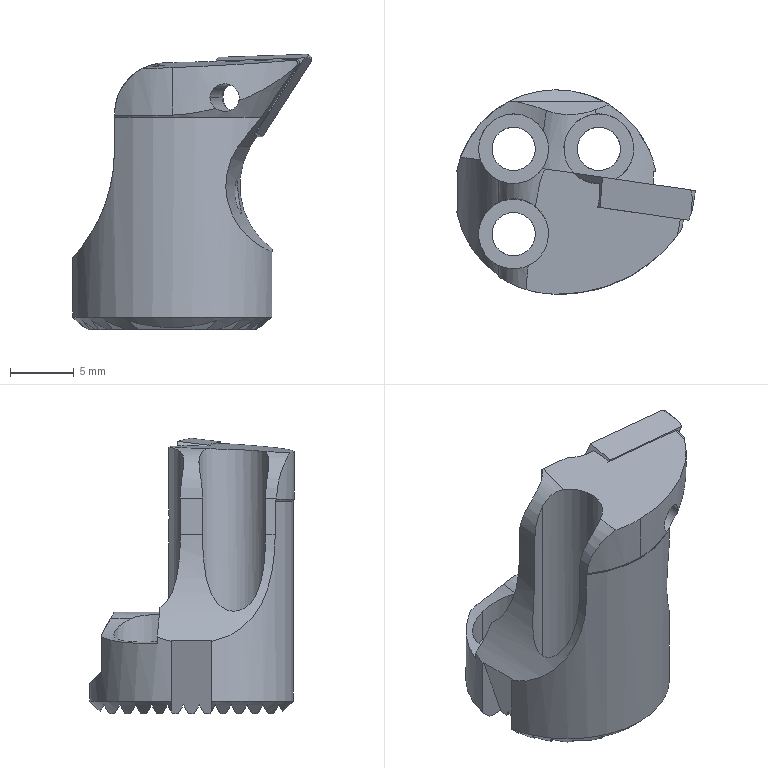Part | 2 solids | 143 faces | volume 1841 mm3 | plane 101 | cylinder 37 | cone 5 | commonest cylinder face diameters 5.5 x7 3.4 x6 2 x2 2.16 x2 2.8 x2 3.5 x2